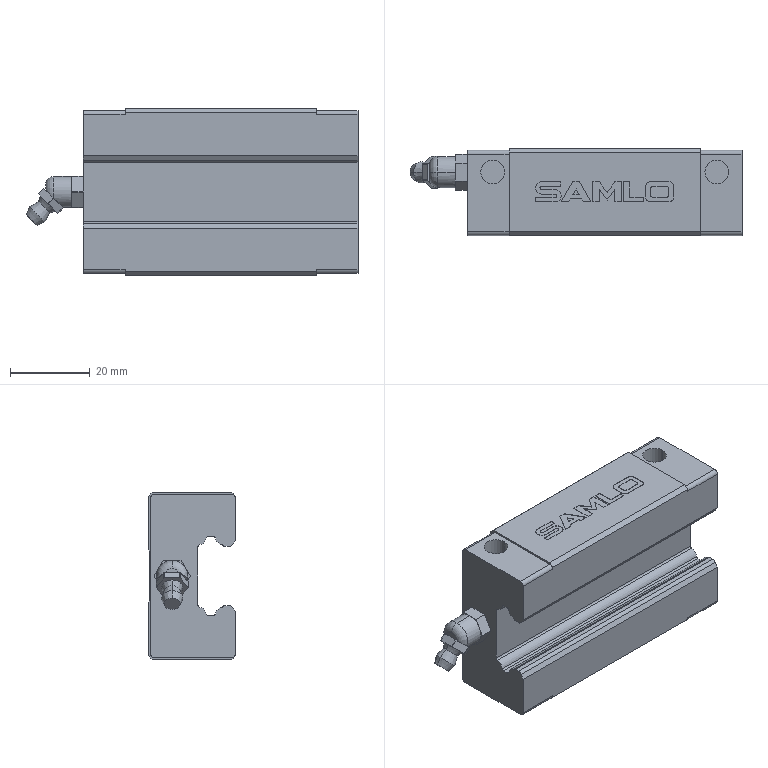Part | SolidWorks | features BaseBody 1 | 1 solid | 203 faces | box 83.53 x 22 x 42 mm | volume 51004 mm3 | plane 119 | cylinder 68 | cone 14 | torus 2 | commonest cylinder face diameters 1 x10 2 x10 4.134 x8 6 x8 8 x6 9 x6